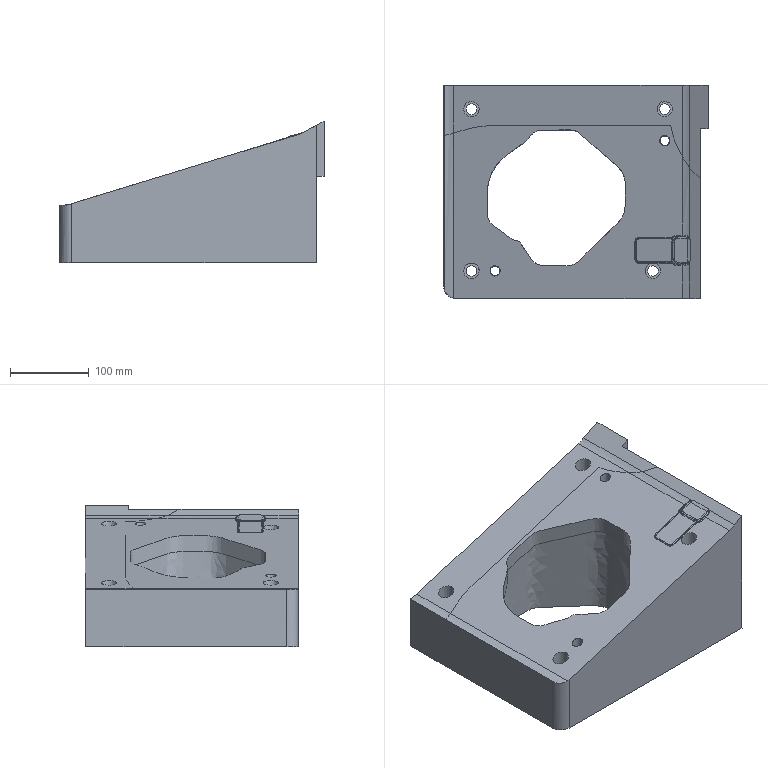Part | NX | features solid 2 | 1 solid | 107 faces | box 335 x 270 x 179.884 mm | volume 7620802 mm3 | spline 80 | plane 14 | cylinder 13 | commonest cylinder face diameters 13.5 x4 19.5 x4 12 x2 13 x2 30 x1